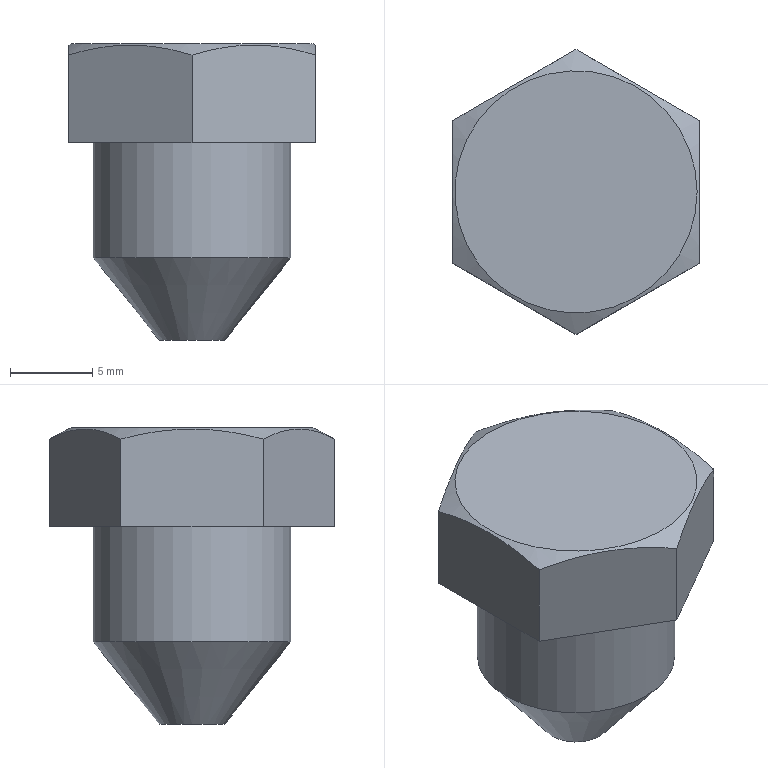Part | STEP file | 1-46.7 | 1 solid | 12 faces | box 15 x 17.321 x 18 mm | volume 2228 mm3 | plane 9 | cone 2 | cylinder 1 | commonest cylinder face diameters 12 x1
STEP:
#1=CARTESIAN_POINT('',(0.,0.,0.));
#2=DIRECTION('',(0.,0.,1.));
#3=DIRECTION('',(1.,0.,0.));
#4=AXIS2_PLACEMENT_3D('',#1,#2,#3);
#5=CARTESIAN_POINT('',(-7.5,-4.33,0.));
#6=VERTEX_POINT('',#5);
#7=CARTESIAN_POINT('',(-7.5,4.33,0.));
#8=VERTEX_POINT('',#7);
#9=CARTESIAN_POINT('',(-7.5,-4.33,0.));
#10=DIRECTION('',(0.,1.,0.));
#11=VECTOR('',#10,1.);
#12=LINE('',#9,#11);
#13=CARTESIAN_POINT('',(1.16,0.,0.));
#14=DIRECTION('',(0.,0.,-1.));
#15=DIRECTION('',(1.,0.,0.));
#16=AXIS2_PLACEMENT_3D('',#13,#14,#15);
#17=PLANE('',#16);
#18=CARTESIAN_POINT('',(-8.66,4.33));
#19=DIRECTION('',(0.,-1.));
#20=VECTOR('',#19,1.);
#21=LINE('',#18,#20);
#22=(GEOMETRIC_REPRESENTATION_CONTEXT(2)PARAMETRIC_REPRESENTATION_CONTEXT()REPRESENTATION_CONTEXT('',''));
#23=DEFINITIONAL_REPRESENTATION('',(#21),#22);
#24=PCURVE('',#17,#23);
#25=CARTESIAN_POINT('',(-7.5,0.,3.));
#26=DIRECTION('',(1.,0.,0.));
#27=DIRECTION('',(0.,1.,0.));
#28=AXIS2_PLACEMENT_3D('',#25,#26,#27);
#29=PLANE('',#28);
#30=CARTESIAN_POINT('',(-4.33,-3.));
#31=DIRECTION('',(1.,0.));
#32=VECTOR('',#31,1.);
#33=LINE('',#30,#32);
#34=(GEOMETRIC_REPRESENTATION_CONTEXT(2)PARAMETRIC_REPRESENTATION_CONTEXT()REPRESENTATION_CONTEXT('',''));
#35=DEFINITIONAL_REPRESENTATION('',(#33),#34);
#36=PCURVE('',#29,#35);
#37=SURFACE_CURVE('',#12,(#24,#36),.PCURVE_S1.);
#38=EDGE_CURVE('',#6,#8,#37,.T.);
#39=ORIENTED_EDGE('',*,*,#38,.T.);
#40=CARTESIAN_POINT('',(0.,8.66,0.));
#41=VERTEX_POINT('',#40);
#42=CARTESIAN_POINT('',(-7.5,4.33,0.));
#43=DIRECTION('',(0.866,0.5,0.));
#44=VECTOR('',#43,1.);
#45=LINE('',#42,#44);
#46=CARTESIAN_POINT('',(-8.66,-4.33));
#47=DIRECTION('',(0.866,-0.5));
#48=VECTOR('',#47,1.);
#49=LINE('',#46,#48);
#50=(GEOMETRIC_REPRESENTATION_CONTEXT(2)PARAMETRIC_REPRESENTATION_CONTEXT()REPRESENTATION_CONTEXT('',''));
#51=DEFINITIONAL_REPRESENTATION('',(#49),#50);
#52=PCURVE('',#17,#51);
#53=CARTESIAN_POINT('',(-3.75,6.495,3.));
#54=DIRECTION('',(0.5,-0.866,0.));
#55=DIRECTION('',(0.866,0.5,0.));
#56=AXIS2_PLACEMENT_3D('',#53,#54,#55);
#57=PLANE('',#56);
#58=CARTESIAN_POINT('',(-4.33,-3.));
#59=DIRECTION('',(1.,0.));
#60=VECTOR('',#59,1.);
#61=LINE('',#58,#60);
#62=(GEOMETRIC_REPRESENTATION_CONTEXT(2)PARAMETRIC_REPRESENTATION_CONTEXT()REPRESENTATION_CONTEXT('',''));
#63=DEFINITIONAL_REPRESENTATION('',(#61),#62);
#64=PCURVE('',#57,#63);
#65=SURFACE_CURVE('',#45,(#52,#64),.PCURVE_S1.);
#66=EDGE_CURVE('',#8,#41,#65,.T.);
#67=ORIENTED_EDGE('',*,*,#66,.T.);
#68=CARTESIAN_POINT('',(7.5,4.33,0.));
#69=VERTEX_POINT('',#68);
#70=CARTESIAN_POINT('',(0.,8.66,0.));
#71=DIRECTION('',(0.866,-0.5,0.));
#72=VECTOR('',#71,1.);
#73=LINE('',#70,#72);
#74=CARTESIAN_POINT('',(-1.16,-8.66));
#75=DIRECTION('',(0.866,0.5));
#76=VECTOR('',#75,1.);
#77=LINE('',#74,#76);
#78=(GEOMETRIC_REPRESENTATION_CONTEXT(2)PARAMETRIC_REPRESENTATION_CONTEXT()REPRESENTATION_CONTEXT('',''));
#79=DEFINITIONAL_REPRESENTATION('',(#77),#78);
#80=PCURVE('',#17,#79);
#81=CARTESIAN_POINT('',(3.75,6.495,3.));
#82=DIRECTION('',(-0.5,-0.866,0.));
#83=DIRECTION('',(0.866,-0.5,0.));
#84=AXIS2_PLACEMENT_3D('',#81,#82,#83);
#85=PLANE('',#84);
#86=CARTESIAN_POINT('',(-4.33,-3.));
#87=DIRECTION('',(1.,0.));
#88=VECTOR('',#87,1.);
#89=LINE('',#86,#88);
#90=(GEOMETRIC_REPRESENTATION_CONTEXT(2)PARAMETRIC_REPRESENTATION_CONTEXT()REPRESENTATION_CONTEXT('',''));
#91=DEFINITIONAL_REPRESENTATION('',(#89),#90);
#92=PCURVE('',#85,#91);
#93=SURFACE_CURVE('',#73,(#80,#92),.PCURVE_S1.);
#94=EDGE_CURVE('',#41,#69,#93,.T.);
#95=ORIENTED_EDGE('',*,*,#94,.T.);
#96=CARTESIAN_POINT('',(7.5,-4.33,0.));
#97=VERTEX_POINT('',#96);
#98=CARTESIAN_POINT('',(7.5,4.33,0.));
#99=DIRECTION('',(0.,-1.,0.));
#100=VECTOR('',#99,1.);
#101=LINE('',#98,#100);
#102=CARTESIAN_POINT('',(6.34,-4.33));
#103=DIRECTION('',(0.,1.));
#104=VECTOR('',#103,1.);
#105=LINE('',#102,#104);
#106=(GEOMETRIC_REPRESENTATION_CONTEXT(2)PARAMETRIC_REPRESENTATION_CONTEXT()REPRESENTATION_CONTEXT('',''));
#107=DEFINITIONAL_REPRESENTATION('',(#105),#106);
#108=PCURVE('',#17,#107);
#109=CARTESIAN_POINT('',(7.5,0.,3.));
#110=DIRECTION('',(-1.,0.,0.));
#111=DIRECTION('',(0.,-1.,0.));
#112=AXIS2_PLACEMENT_3D('',#109,#110,#111);
#113=PLANE('',#112);
#114=CARTESIAN_POINT('',(-4.33,-3.));
#115=DIRECTION('',(1.,0.));
#116=VECTOR('',#115,1.);
#117=LINE('',#114,#116);
#118=(GEOMETRIC_REPRESENTATION_CONTEXT(2)PARAMETRIC_REPRESENTATION_CONTEXT()REPRESENTATION_CONTEXT('',''));
#119=DEFINITIONAL_REPRESENTATION('',(#117),#118);
#120=PCURVE('',#113,#119);
#121=SURFACE_CURVE('',#101,(#108,#120),.PCURVE_S1.);
#122=EDGE_CURVE('',#69,#97,#121,.T.);
#123=ORIENTED_EDGE('',*,*,#122,.T.);
#124=CARTESIAN_POINT('',(0.,-8.66,0.));
#125=VERTEX_POINT('',#124);
#126=CARTESIAN_POINT('',(7.5,-4.33,0.));
#127=DIRECTION('',(-0.866,-0.5,0.));
#128=VECTOR('',#127,1.);
#129=LINE('',#126,#128);
#130=CARTESIAN_POINT('',(6.34,4.33));
#131=DIRECTION('',(-0.866,0.5));
#132=VECTOR('',#131,1.);
#133=LINE('',#130,#132);
#134=(GEOMETRIC_REPRESENTATION_CONTEXT(2)PARAMETRIC_REPRESENTATION_CONTEXT()REPRESENTATION_CONTEXT('',''));
#135=DEFINITIONAL_REPRESENTATION('',(#133),#134);
#136=PCURVE('',#17,#135);
#137=CARTESIAN_POINT('',(3.75,-6.495,3.));
#138=DIRECTION('',(-0.5,0.866,0.));
#139=DIRECTION('',(-0.866,-0.5,0.));
#140=AXIS2_PLACEMENT_3D('',#137,#138,#139);
#141=PLANE('',#140);
#142=CARTESIAN_POINT('',(-4.33,-3.));
#143=DIRECTION('',(1.,0.));
#144=VECTOR('',#143,1.);
#145=LINE('',#142,#144);
#146=(GEOMETRIC_REPRESENTATION_CONTEXT(2)PARAMETRIC_REPRESENTATION_CONTEXT()REPRESENTATION_CONTEXT('',''));
#147=DEFINITIONAL_REPRESENTATION('',(#145),#146);
#148=PCURVE('',#141,#147);
#149=SURFACE_CURVE('',#129,(#136,#148),.PCURVE_S1.);
#150=EDGE_CURVE('',#97,#125,#149,.T.);
#151=ORIENTED_EDGE('',*,*,#150,.T.);
#152=CARTESIAN_POINT('',(0.,-8.66,0.));
#153=DIRECTION('',(-0.866,0.5,0.));
#154=VECTOR('',#153,1.);
#155=LINE('',#152,#154);
#156=CARTESIAN_POINT('',(-1.16,8.66));
#157=DIRECTION('',(-0.866,-0.5));
#158=VECTOR('',#157,1.);
#159=LINE('',#156,#158);
#160=(GEOMETRIC_REPRESENTATION_CONTEXT(2)PARAMETRIC_REPRESENTATION_CONTEXT()REPRESENTATION_CONTEXT('',''));
#161=DEFINITIONAL_REPRESENTATION('',(#159),#160);
#162=PCURVE('',#17,#161);
#163=CARTESIAN_POINT('',(-3.75,-6.495,3.));
#164=DIRECTION('',(0.5,0.866,0.));
#165=DIRECTION('',(-0.866,0.5,0.));
#166=AXIS2_PLACEMENT_3D('',#163,#164,#165);
#167=PLANE('',#166);
#168=CARTESIAN_POINT('',(-4.33,-3.));
#169=DIRECTION('',(1.,0.));
#170=VECTOR('',#169,1.);
#171=LINE('',#168,#170);
#172=(GEOMETRIC_REPRESENTATION_CONTEXT(2)PARAMETRIC_REPRESENTATION_CONTEXT()REPRESENTATION_CONTEXT('',''));
#173=DEFINITIONAL_REPRESENTATION('',(#171),#172);
#174=PCURVE('',#167,#173);
#175=SURFACE_CURVE('',#155,(#162,#174),.PCURVE_S1.);
#176=EDGE_CURVE('',#125,#6,#175,.T.);
#177=ORIENTED_EDGE('',*,*,#176,.T.);
#178=EDGE_LOOP('',(#39,#67,#95,#123,#151,#177));
#179=FACE_BOUND('',#178,.T.);
#180=CARTESIAN_POINT('',(0.,6.,0.));
#181=VERTEX_POINT('',#180);
#182=CARTESIAN_POINT('',(0.,0.,0.));
#183=DIRECTION('',(0.,0.,1.));
#184=DIRECTION('',(0.,1.,0.));
#185=AXIS2_PLACEMENT_3D('',#182,#183,#184);
#186=CIRCLE('',#185,6.);
#187=CARTESIAN_POINT('',(-1.16,-6.));
#188=CARTESIAN_POINT('',(-11.553,-6.));
#189=CARTESIAN_POINT('',(-6.356,3.));
#190=CARTESIAN_POINT('',(-1.16,12.));
#191=CARTESIAN_POINT('',(4.036,3.));
#192=CARTESIAN_POINT('',(9.232,-6.));
#193=CARTESIAN_POINT('',(-1.16,-6.));
#194=(BOUNDED_CURVE()B_SPLINE_CURVE(2,(#187,#188,#189,#190,#191,#192,#193),.UNSPECIFIED.,.T.,.F.)B_SPLINE_CURVE_WITH_KNOTS((1,2,2,2,2,1),(-2.094,0.,2.094,4.189,6.283,8.378),.UNSPECIFIED.)CURVE()GEOMETRIC_REPRESENTATION_ITEM()RATIONAL_B_SPLINE_CURVE((1.,0.5,1.,0.5,1.,0.5,1.))REPRESENTATION_ITEM(''));
#195=(GEOMETRIC_REPRESENTATION_CONTEXT(2)PARAMETRIC_REPRESENTATION_CONTEXT()REPRESENTATION_CONTEXT('',''));
#196=DEFINITIONAL_REPRESENTATION('',(#194),#195);
#197=PCURVE('',#17,#196);
#198=CARTESIAN_POINT('',(0.,0.,0.));
#199=DIRECTION('',(0.,0.,-1.));
#200=DIRECTION('',(0.,1.,0.));
#201=AXIS2_PLACEMENT_3D('',#198,#199,#200);
#202=CYLINDRICAL_SURFACE('',#201,6.);
#203=CARTESIAN_POINT('',(6.283,0.));
#204=DIRECTION('',(-1.,0.));
#205=VECTOR('',#204,1.);
#206=LINE('',#203,#205);
#207=(GEOMETRIC_REPRESENTATION_CONTEXT(2)PARAMETRIC_REPRESENTATION_CONTEXT()REPRESENTATION_CONTEXT('',''));
#208=DEFINITIONAL_REPRESENTATION('',(#206),#207);
#209=PCURVE('',#202,#208);
#210=SURFACE_CURVE('',#186,(#197,#209),.PCURVE_S1.);
#211=EDGE_CURVE('',#181,#181,#210,.T.);
#212=ORIENTED_EDGE('',*,*,#211,.T.);
#213=EDGE_LOOP('',(#212));
#214=FACE_BOUND('',#213,.T.);
#215=ADVANCED_FACE('',(#179,#214),#17,.T.);
#216=CARTESIAN_POINT('',(0.,6.,-7.));
#217=VERTEX_POINT('',#216);
#218=CARTESIAN_POINT('',(0.,6.,0.));
#219=DIRECTION('',(0.,0.,-1.));
#220=VECTOR('',#219,1.);
#221=LINE('',#218,#220);
#222=CARTESIAN_POINT('',(6.283,0.));
#223=DIRECTION('',(0.,1.));
#224=VECTOR('',#223,1.);
#225=LINE('',#222,#224);
#226=(GEOMETRIC_REPRESENTATION_CONTEXT(2)PARAMETRIC_REPRESENTATION_CONTEXT()REPRESENTATION_CONTEXT('',''));
#227=DEFINITIONAL_REPRESENTATION('',(#225),#226);
#228=PCURVE('',#202,#227);
#229=CARTESIAN_POINT('',(0.,0.));
#230=DIRECTION('',(0.,1.));
#231=VECTOR('',#230,1.);
#232=LINE('',#229,#231);
#233=(GEOMETRIC_REPRESENTATION_CONTEXT(2)PARAMETRIC_REPRESENTATION_CONTEXT()REPRESENTATION_CONTEXT('',''));
#234=DEFINITIONAL_REPRESENTATION('',(#232),#233);
#235=PCURVE('',#202,#234);
#236=SEAM_CURVE('',#221,(#228,#235),.PCURVE_S1.);
#237=EDGE_CURVE('',#181,#217,#236,.T.);
#238=ORIENTED_EDGE('',*,*,#237,.T.);
#239=CARTESIAN_POINT('',(6.,0.,-7.));
#240=VERTEX_POINT('',#239);
#241=CARTESIAN_POINT('',(0.,0.,-7.));
#242=DIRECTION('',(0.,0.,1.));
#243=DIRECTION('',(0.,1.,0.));
#244=AXIS2_PLACEMENT_3D('',#241,#242,#243);
#245=CIRCLE('',#244,6.);
#246=CARTESIAN_POINT('',(6.283,7.));
#247=DIRECTION('',(-1.,0.));
#248=VECTOR('',#247,1.);
#249=LINE('',#246,#248);
#250=(GEOMETRIC_REPRESENTATION_CONTEXT(2)PARAMETRIC_REPRESENTATION_CONTEXT()REPRESENTATION_CONTEXT('',''));
#251=DEFINITIONAL_REPRESENTATION('',(#249),#250);
#252=PCURVE('',#202,#251);
#253=CARTESIAN_POINT('',(0.,0.,-12.));
#254=DIRECTION('',(0.,0.,1.));
#255=DIRECTION('',(1.,0.,0.));
#256=AXIS2_PLACEMENT_3D('',#253,#254,#255);
#257=CONICAL_SURFACE('',#256,2.,0.6747);
#258=CARTESIAN_POINT('',(1.571,5.));
#259=DIRECTION('',(1.,0.));
#260=VECTOR('',#259,1.);
#261=LINE('',#258,#260);
#262=(GEOMETRIC_REPRESENTATION_CONTEXT(2)PARAMETRIC_REPRESENTATION_CONTEXT()REPRESENTATION_CONTEXT('',''));
#263=DEFINITIONAL_REPRESENTATION('',(#261),#262);
#264=PCURVE('',#257,#263);
#265=SURFACE_CURVE('',#245,(#252,#264),.PCURVE_S1.);
#266=EDGE_CURVE('',#217,#240,#265,.T.);
#267=ORIENTED_EDGE('',*,*,#266,.T.);
#268=CARTESIAN_POINT('',(0.,0.,-7.));
#269=DIRECTION('',(0.,0.,1.));
#270=DIRECTION('',(1.,0.,0.));
#271=AXIS2_PLACEMENT_3D('',#268,#269,#270);
#272=CIRCLE('',#271,6.);
#273=CARTESIAN_POINT('',(1.571,7.));
#274=DIRECTION('',(-1.,0.));
#275=VECTOR('',#274,1.);
#276=LINE('',#273,#275);
#277=(GEOMETRIC_REPRESENTATION_CONTEXT(2)PARAMETRIC_REPRESENTATION_CONTEXT()REPRESENTATION_CONTEXT('',''));
#278=DEFINITIONAL_REPRESENTATION('',(#276),#277);
#279=PCURVE('',#202,#278);
#280=CARTESIAN_POINT('',(0.,5.));
#281=DIRECTION('',(1.,0.));
#282=VECTOR('',#281,1.);
#283=LINE('',#280,#282);
#284=(GEOMETRIC_REPRESENTATION_CONTEXT(2)PARAMETRIC_REPRESENTATION_CONTEXT()REPRESENTATION_CONTEXT('',''));
#285=DEFINITIONAL_REPRESENTATION('',(#283),#284);
#286=PCURVE('',#257,#285);
#287=SURFACE_CURVE('',#272,(#279,#286),.PCURVE_S1.);
#288=EDGE_CURVE('',#240,#217,#287,.T.);
#289=ORIENTED_EDGE('',*,*,#288,.T.);
#290=ORIENTED_EDGE('',*,*,#237,.F.);
#291=ORIENTED_EDGE('',*,*,#211,.F.);
#292=EDGE_LOOP('',(#238,#267,#289,#290,#291));
#293=FACE_BOUND('',#292,.T.);
#294=ADVANCED_FACE('',(#293),#202,.T.);
#295=CARTESIAN_POINT('',(2.,0.,-12.));
#296=VERTEX_POINT('',#295);
#297=CARTESIAN_POINT('',(0.,0.,-12.));
#298=DIRECTION('',(0.,0.,1.));
#299=DIRECTION('',(1.,0.,0.));
#300=AXIS2_PLACEMENT_3D('',#297,#298,#299);
#301=CIRCLE('',#300,2.);
#302=CARTESIAN_POINT('',(0.,0.));
#303=DIRECTION('',(1.,0.));
#304=VECTOR('',#303,1.);
#305=LINE('',#302,#304);
#306=(GEOMETRIC_REPRESENTATION_CONTEXT(2)PARAMETRIC_REPRESENTATION_CONTEXT()REPRESENTATION_CONTEXT('',''));
#307=DEFINITIONAL_REPRESENTATION('',(#305),#306);
#308=PCURVE('',#257,#307);
#309=CARTESIAN_POINT('',(0.,0.,-12.));
#310=DIRECTION('',(0.,0.,1.));
#311=DIRECTION('',(1.,0.,0.));
#312=AXIS2_PLACEMENT_3D('',#309,#310,#311);
#313=PLANE('',#312);
#314=CARTESIAN_POINT('',(0.,0.));
#315=DIRECTION('',(1.,0.));
#316=AXIS2_PLACEMENT_2D('',#314,#315);
#317=CIRCLE('',#316,2.);
#318=(GEOMETRIC_REPRESENTATION_CONTEXT(2)PARAMETRIC_REPRESENTATION_CONTEXT()REPRESENTATION_CONTEXT('',''));
#319=DEFINITIONAL_REPRESENTATION('',(#317),#318);
#320=PCURVE('',#313,#319);
#321=SURFACE_CURVE('',#301,(#308,#320),.PCURVE_S1.);
#322=EDGE_CURVE('',#296,#296,#321,.T.);
#323=ORIENTED_EDGE('',*,*,#322,.T.);
#324=CARTESIAN_POINT('',(2.,0.,-12.));
#325=DIRECTION('',(0.6247,0.,0.7809));
#326=VECTOR('',#325,1.);
#327=LINE('',#324,#326);
#328=CARTESIAN_POINT('',(6.283,0.));
#329=DIRECTION('',(0.,1.));
#330=VECTOR('',#329,1.);
#331=LINE('',#328,#330);
#332=(GEOMETRIC_REPRESENTATION_CONTEXT(2)PARAMETRIC_REPRESENTATION_CONTEXT()REPRESENTATION_CONTEXT('',''));
#333=DEFINITIONAL_REPRESENTATION('',(#331),#332);
#334=PCURVE('',#257,#333);
#335=CARTESIAN_POINT('',(0.,0.));
#336=DIRECTION('',(0.,1.));
#337=VECTOR('',#336,1.);
#338=LINE('',#335,#337);
#339=(GEOMETRIC_REPRESENTATION_CONTEXT(2)PARAMETRIC_REPRESENTATION_CONTEXT()REPRESENTATION_CONTEXT('',''));
#340=DEFINITIONAL_REPRESENTATION('',(#338),#339);
#341=PCURVE('',#257,#340);
#342=SEAM_CURVE('',#327,(#334,#341),.PCURVE_S1.);
#343=EDGE_CURVE('',#296,#240,#342,.T.);
#344=ORIENTED_EDGE('',*,*,#343,.T.);
#345=ORIENTED_EDGE('',*,*,#266,.F.);
#346=ORIENTED_EDGE('',*,*,#288,.F.);
#347=ORIENTED_EDGE('',*,*,#343,.F.);
#348=EDGE_LOOP('',(#323,#344,#345,#346,#347));
#349=FACE_BOUND('',#348,.T.);
#350=ADVANCED_FACE('',(#349),#257,.T.);
#351=ORIENTED_EDGE('',*,*,#322,.T.);
#352=EDGE_LOOP('',(#351));
#353=FACE_BOUND('',#352,.F.);
#354=ADVANCED_FACE('',(#353),#313,.F.);
#355=CARTESIAN_POINT('',(7.357,0.,6.));
#356=VERTEX_POINT('',#355);
#357=CARTESIAN_POINT('',(0.,0.,6.));
#358=DIRECTION('',(0.,0.,1.));
#359=DIRECTION('',(1.,0.,0.));
#360=AXIS2_PLACEMENT_3D('',#357,#358,#359);
#361=CIRCLE('',#360,7.357);
#362=CARTESIAN_POINT('',(1.16,0.,6.));
#363=DIRECTION('',(0.,0.,-1.));
#364=DIRECTION('',(1.,0.,0.));
#365=AXIS2_PLACEMENT_3D('',#362,#363,#364);
#366=PLANE('',#365);
#367=CARTESIAN_POINT('',(6.197,0.));
#368=CARTESIAN_POINT('',(6.197,-12.743));
#369=CARTESIAN_POINT('',(-4.839,-6.371));
#370=CARTESIAN_POINT('',(-15.874,0.));
#371=CARTESIAN_POINT('',(-4.839,6.371));
#372=CARTESIAN_POINT('',(6.197,12.743));
#373=CARTESIAN_POINT('',(6.197,0.));
#374=(BOUNDED_CURVE()B_SPLINE_CURVE(2,(#367,#368,#369,#370,#371,#372,#373),.UNSPECIFIED.,.T.,.F.)B_SPLINE_CURVE_WITH_KNOTS((1,2,2,2,2,1),(-2.094,0.,2.094,4.189,6.283,8.378),.UNSPECIFIED.)CURVE()GEOMETRIC_REPRESENTATION_ITEM()RATIONAL_B_SPLINE_CURVE((1.,0.5,1.,0.5,1.,0.5,1.))REPRESENTATION_ITEM(''));
#375=(GEOMETRIC_REPRESENTATION_CONTEXT(2)PARAMETRIC_REPRESENTATION_CONTEXT()REPRESENTATION_CONTEXT('',''));
#376=DEFINITIONAL_REPRESENTATION('',(#374),#375);
#377=PCURVE('',#366,#376);
#378=CARTESIAN_POINT('',(0.,0.,6.));
#379=DIRECTION('',(0.,0.,-1.));
#380=DIRECTION('',(1.,0.,0.));
#381=AXIS2_PLACEMENT_3D('',#378,#379,#380);
#382=CONICAL_SURFACE('',#381,7.357,1.09);
#383=CARTESIAN_POINT('',(6.283,0.));
#384=DIRECTION('',(-1.,0.));
#385=VECTOR('',#384,1.);
#386=LINE('',#383,#385);
#387=(GEOMETRIC_REPRESENTATION_CONTEXT(2)PARAMETRIC_REPRESENTATION_CONTEXT()REPRESENTATION_CONTEXT('',''));
#388=DEFINITIONAL_REPRESENTATION('',(#386),#387);
#389=PCURVE('',#382,#388);
#390=SURFACE_CURVE('',#361,(#377,#389),.PCURVE_S1.);
#391=EDGE_CURVE('',#356,#356,#390,.T.);
#392=ORIENTED_EDGE('',*,*,#391,.F.);
#393=EDGE_LOOP('',(#392));
#394=FACE_BOUND('',#393,.F.);
#395=ADVANCED_FACE('',(#394),#366,.F.);
#396=ORIENTED_EDGE('',*,*,#38,.T.);
#397=CARTESIAN_POINT('',(-7.5,4.33,5.32));
#398=VERTEX_POINT('',#397);
#399=CARTESIAN_POINT('',(-7.5,4.33,0.));
#400=DIRECTION('',(0.,0.,1.));
#401=VECTOR('',#400,1.);
#402=LINE('',#399,#401);
#403=CARTESIAN_POINT('',(4.33,-3.));
#404=DIRECTION('',(0.,1.));
#405=VECTOR('',#404,1.);
#406=LINE('',#403,#405);
#407=(GEOMETRIC_REPRESENTATION_CONTEXT(2)PARAMETRIC_REPRESENTATION_CONTEXT()REPRESENTATION_CONTEXT('',''));
#408=DEFINITIONAL_REPRESENTATION('',(#406),#407);
#409=PCURVE('',#29,#408);
#410=CARTESIAN_POINT('',(-4.33,-3.));
#411=DIRECTION('',(0.,1.));
#412=VECTOR('',#411,1.);
#413=LINE('',#410,#412);
#414=(GEOMETRIC_REPRESENTATION_CONTEXT(2)PARAMETRIC_REPRESENTATION_CONTEXT()REPRESENTATION_CONTEXT('',''));
#415=DEFINITIONAL_REPRESENTATION('',(#413),#414);
#416=PCURVE('',#57,#415);
#417=SURFACE_CURVE('',#402,(#409,#416),.PCURVE_S1.);
#418=EDGE_CURVE('',#8,#398,#417,.T.);
#419=ORIENTED_EDGE('',*,*,#418,.T.);
#420=CARTESIAN_POINT('',(-7.5,-4.33,5.32));
#421=VERTEX_POINT('',#420);
#422=CARTESIAN_POINT('',(-7.5,4.33,5.32));
#423=CARTESIAN_POINT('',(-7.5,0.,6.45));
#424=CARTESIAN_POINT('',(-7.5,-4.33,5.32));
#425=(BOUNDED_CURVE()B_SPLINE_CURVE(2,(#422,#423,#424),.UNSPECIFIED.,.F.,.F.)B_SPLINE_CURVE_WITH_KNOTS((3,3),(0.,1.),.PIECEWISE_BEZIER_KNOTS.)CURVE()GEOMETRIC_REPRESENTATION_ITEM()RATIONAL_B_SPLINE_CURVE((1.631,1.883,1.631))REPRESENTATION_ITEM(''));
#426=CARTESIAN_POINT('',(4.33,2.32));
#427=CARTESIAN_POINT('',(0.,3.45));
#428=CARTESIAN_POINT('',(-4.33,2.32));
#429=(BOUNDED_CURVE()B_SPLINE_CURVE(2,(#426,#427,#428),.UNSPECIFIED.,.F.,.F.)B_SPLINE_CURVE_WITH_KNOTS((3,3),(0.,1.),.PIECEWISE_BEZIER_KNOTS.)CURVE()GEOMETRIC_REPRESENTATION_ITEM()RATIONAL_B_SPLINE_CURVE((1.631,1.883,1.631))REPRESENTATION_ITEM(''));
#430=(GEOMETRIC_REPRESENTATION_CONTEXT(2)PARAMETRIC_REPRESENTATION_CONTEXT()REPRESENTATION_CONTEXT('',''));
#431=DEFINITIONAL_REPRESENTATION('',(#429),#430);
#432=PCURVE('',#29,#431);
#433=CARTESIAN_POINT('',(3.665,0.6804));
#434=CARTESIAN_POINT('',(3.65,0.6409));
#435=CARTESIAN_POINT('',(3.62,0.5665));
#436=CARTESIAN_POINT('',(3.573,0.468));
#437=CARTESIAN_POINT('',(3.527,0.3819));
#438=CARTESIAN_POINT('',(3.479,0.3074));
#439=CARTESIAN_POINT('',(3.432,0.2439));
#440=CARTESIAN_POINT('',(3.384,0.1909));
#441=CARTESIAN_POINT('',(3.336,0.1481));
#442=CARTESIAN_POINT('',(3.288,0.1151));
#443=CARTESIAN_POINT('',(3.239,0.09176));
#444=CARTESIAN_POINT('',(3.19,0.07779));
#445=CARTESIAN_POINT('',(3.142,0.07315));
#446=CARTESIAN_POINT('',(3.093,0.07779));
#447=CARTESIAN_POINT('',(3.044,0.09176));
#448=CARTESIAN_POINT('',(2.996,0.1151));
#449=CARTESIAN_POINT('',(2.947,0.1481));
#450=CARTESIAN_POINT('',(2.899,0.1909));
#451=CARTESIAN_POINT('',(2.851,0.2439));
#452=CARTESIAN_POINT('',(2.804,0.3074));
#453=CARTESIAN_POINT('',(2.757,0.3819));
#454=CARTESIAN_POINT('',(2.71,0.468));
#455=CARTESIAN_POINT('',(2.664,0.5665));
#456=CARTESIAN_POINT('',(2.633,0.6409));
#457=CARTESIAN_POINT('',(2.618,0.6804));
#458=B_SPLINE_CURVE_WITH_KNOTS('',3,(#433,#434,#435,#436,#437,#438,#439,#440,#441,#442,#443,#444,#445,#446,#447,#448,#449,#450,#451,#452,#453,#454,#455,#456,#457),.UNSPECIFIED.,.F.,.F.,(4,1,1,1,1,1,1,1,1,1,1,1,1,1,1,1,1,1,1,1,1,1,4),(0.,0.04545,0.09091,0.1364,0.1818,0.2273,0.2727,0.3182,0.3636,0.4091,0.4545,0.5,0.5455,0.5909,0.6364,0.6818,0.7273,0.7727,0.8182,0.8636,0.9091,0.9545,1.),.QUASI_UNIFORM_KNOTS.);
#459=(GEOMETRIC_REPRESENTATION_CONTEXT(2)PARAMETRIC_REPRESENTATION_CONTEXT()REPRESENTATION_CONTEXT('',''));
#460=DEFINITIONAL_REPRESENTATION('',(#458),#459);
#461=PCURVE('',#382,#460);
#462=SURFACE_CURVE('',#425,(#432,#461),.PCURVE_S1.);
#463=EDGE_CURVE('',#398,#421,#462,.T.);
#464=ORIENTED_EDGE('',*,*,#463,.T.);
#465=CARTESIAN_POINT('',(-7.5,-4.33,0.));
#466=DIRECTION('',(0.,0.,1.));
#467=VECTOR('',#466,1.);
#468=LINE('',#465,#467);
#469=CARTESIAN_POINT('',(-4.33,-3.));
#470=DIRECTION('',(0.,1.));
#471=VECTOR('',#470,1.);
#472=LINE('',#469,#471);
#473=(GEOMETRIC_REPRESENTATION_CONTEXT(2)PARAMETRIC_REPRESENTATION_CONTEXT()REPRESENTATION_CONTEXT('',''));
#474=DEFINITIONAL_REPRESENTATION('',(#472),#473);
#475=PCURVE('',#29,#474);
#476=CARTESIAN_POINT('',(4.33,-3.));
#477=DIRECTION('',(0.,1.));
#478=VECTOR('',#477,1.);
#479=LINE('',#476,#478);
#480=(GEOMETRIC_REPRESENTATION_CONTEXT(2)PARAMETRIC_REPRESENTATION_CONTEXT()REPRESENTATION_CONTEXT('',''));
#481=DEFINITIONAL_REPRESENTATION('',(#479),#480);
#482=PCURVE('',#167,#481);
#483=SURFACE_CURVE('',#468,(#475,#482),.PCURVE_S1.);
#484=EDGE_CURVE('',#6,#421,#483,.T.);
#485=ORIENTED_EDGE('',*,*,#484,.F.);
#486=EDGE_LOOP('',(#396,#419,#464,#485));
#487=FACE_BOUND('',#486,.F.);
#488=ADVANCED_FACE('',(#487),#29,.F.);
#489=ORIENTED_EDGE('',*,*,#66,.T.);
#490=CARTESIAN_POINT('',(0.,8.66,5.32));
#491=VERTEX_POINT('',#490);
#492=CARTESIAN_POINT('',(0.,8.66,0.));
#493=DIRECTION('',(0.,0.,1.));
#494=VECTOR('',#493,1.);
#495=LINE('',#492,#494);
#496=CARTESIAN_POINT('',(4.33,-3.));
#497=DIRECTION('',(0.,1.));
#498=VECTOR('',#497,1.);
#499=LINE('',#496,#498);
#500=(GEOMETRIC_REPRESENTATION_CONTEXT(2)PARAMETRIC_REPRESENTATION_CONTEXT()REPRESENTATION_CONTEXT('',''));
#501=DEFINITIONAL_REPRESENTATION('',(#499),#500);
#502=PCURVE('',#57,#501);
#503=CARTESIAN_POINT('',(-4.33,-3.));
#504=DIRECTION('',(0.,1.));
#505=VECTOR('',#504,1.);
#506=LINE('',#503,#505);
#507=(GEOMETRIC_REPRESENTATION_CONTEXT(2)PARAMETRIC_REPRESENTATION_CONTEXT()REPRESENTATION_CONTEXT('',''));
#508=DEFINITIONAL_REPRESENTATION('',(#506),#507);
#509=PCURVE('',#85,#508);
#510=SURFACE_CURVE('',#495,(#502,#509),.PCURVE_S1.);
#511=EDGE_CURVE('',#41,#491,#510,.T.);
#512=ORIENTED_EDGE('',*,*,#511,.T.);
#513=CARTESIAN_POINT('',(0.,8.66,5.32));
#514=CARTESIAN_POINT('',(-3.75,6.495,6.45));
#515=CARTESIAN_POINT('',(-7.5,4.33,5.32));
#516=(BOUNDED_CURVE()B_SPLINE_CURVE(2,(#513,#514,#515),.UNSPECIFIED.,.F.,.F.)B_SPLINE_CURVE_WITH_KNOTS((3,3),(0.,1.),.PIECEWISE_BEZIER_KNOTS.)CURVE()GEOMETRIC_REPRESENTATION_ITEM()RATIONAL_B_SPLINE_CURVE((1.631,1.883,1.631))REPRESENTATION_ITEM(''));
#517=CARTESIAN_POINT('',(4.33,2.32));
#518=CARTESIAN_POINT('',(0.,3.45));
#519=CARTESIAN_POINT('',(-4.33,2.32));
#520=(BOUNDED_CURVE()B_SPLINE_CURVE(2,(#517,#518,#519),.UNSPECIFIED.,.F.,.F.)B_SPLINE_CURVE_WITH_KNOTS((3,3),(0.,1.),.PIECEWISE_BEZIER_KNOTS.)CURVE()GEOMETRIC_REPRESENTATION_ITEM()RATIONAL_B_SPLINE_CURVE((1.631,1.883,1.631))REPRESENTATION_ITEM(''));
#521=(GEOMETRIC_REPRESENTATION_CONTEXT(2)PARAMETRIC_REPRESENTATION_CONTEXT()REPRESENTATION_CONTEXT('',''));
#522=DEFINITIONAL_REPRESENTATION('',(#520),#521);
#523=PCURVE('',#57,#522);
#524=CARTESIAN_POINT('',(4.712,0.6804));
#525=CARTESIAN_POINT('',(4.697,0.6409));
#526=CARTESIAN_POINT('',(4.667,0.5665));
#527=CARTESIAN_POINT('',(4.621,0.468));
#528=CARTESIAN_POINT('',(4.574,0.3819));
#529=CARTESIAN_POINT('',(4.527,0.3074));
#530=CARTESIAN_POINT('',(4.479,0.2439));
#531=CARTESIAN_POINT('',(4.431,0.1909));
#532=CARTESIAN_POINT('',(4.383,0.1481));
#533=CARTESIAN_POINT('',(4.335,0.1151));
#534=CARTESIAN_POINT('',(4.286,0.09176));
#535=CARTESIAN_POINT('',(4.238,0.07779));
#536=CARTESIAN_POINT('',(4.189,0.07315));
#537=CARTESIAN_POINT('',(4.14,0.07779));
#538=CARTESIAN_POINT('',(4.091,0.09176));
#539=CARTESIAN_POINT('',(4.043,0.1151));
#540=CARTESIAN_POINT('',(3.994,0.1481));
#541=CARTESIAN_POINT('',(3.946,0.1909));
#542=CARTESIAN_POINT('',(3.898,0.2439));
#543=CARTESIAN_POINT('',(3.851,0.3074));
#544=CARTESIAN_POINT('',(3.804,0.3819));
#545=CARTESIAN_POINT('',(3.757,0.468));
#546=CARTESIAN_POINT('',(3.711,0.5665));
#547=CARTESIAN_POINT('',(3.68,0.6409));
#548=CARTESIAN_POINT('',(3.665,0.6804));
#549=B_SPLINE_CURVE_WITH_KNOTS('',3,(#524,#525,#526,#527,#528,#529,#530,#531,#532,#533,#534,#535,#536,#537,#538,#539,#540,#541,#542,#543,#544,#545,#546,#547,#548),.UNSPECIFIED.,.F.,.F.,(4,1,1,1,1,1,1,1,1,1,1,1,1,1,1,1,1,1,1,1,1,1,4),(0.,0.04545,0.09091,0.1364,0.1818,0.2273,0.2727,0.3182,0.3636,0.4091,0.4545,0.5,0.5455,0.5909,0.6364,0.6818,0.7273,0.7727,0.8182,0.8636,0.9091,0.9545,1.),.QUASI_UNIFORM_KNOTS.);
#550=(GEOMETRIC_REPRESENTATION_CONTEXT(2)PARAMETRIC_REPRESENTATION_CONTEXT()REPRESENTATION_CONTEXT('',''));
#551=DEFINITIONAL_REPRESENTATION('',(#549),#550);
#552=PCURVE('',#382,#551);
#553=SURFACE_CURVE('',#516,(#523,#552),.PCURVE_S1.);
#554=EDGE_CURVE('',#491,#398,#553,.T.);
#555=ORIENTED_EDGE('',*,*,#554,.T.);
#556=ORIENTED_EDGE('',*,*,#418,.F.);
#557=EDGE_LOOP('',(#489,#512,#555,#556));
#558=FACE_BOUND('',#557,.F.);
#559=ADVANCED_FACE('',(#558),#57,.F.);
#560=ORIENTED_EDGE('',*,*,#94,.T.);
#561=CARTESIAN_POINT('',(7.5,4.33,5.32));
#562=VERTEX_POINT('',#561);
#563=CARTESIAN_POINT('',(7.5,4.33,0.));
#564=DIRECTION('',(0.,0.,1.));
#565=VECTOR('',#564,1.);
#566=LINE('',#563,#565);
#567=CARTESIAN_POINT('',(4.33,-3.));
#568=DIRECTION('',(0.,1.));
#569=VECTOR('',#568,1.);
#570=LINE('',#567,#569);
#571=(GEOMETRIC_REPRESENTATION_CONTEXT(2)PARAMETRIC_REPRESENTATION_CONTEXT()REPRESENTATION_CONTEXT('',''));
#572=DEFINITIONAL_REPRESENTATION('',(#570),#571);
#573=PCURVE('',#85,#572);
#574=CARTESIAN_POINT('',(-4.33,-3.));
#575=DIRECTION('',(0.,1.));
#576=VECTOR('',#575,1.);
#577=LINE('',#574,#576);
#578=(GEOMETRIC_REPRESENTATION_CONTEXT(2)PARAMETRIC_REPRESENTATION_CONTEXT()REPRESENTATION_CONTEXT('',''));
#579=DEFINITIONAL_REPRESENTATION('',(#577),#578);
#580=PCURVE('',#113,#579);
#581=SURFACE_CURVE('',#566,(#573,#580),.PCURVE_S1.);
#582=EDGE_CURVE('',#69,#562,#581,.T.);
#583=ORIENTED_EDGE('',*,*,#582,.T.);
#584=CARTESIAN_POINT('',(7.5,4.33,5.32));
#585=CARTESIAN_POINT('',(3.75,6.495,6.45));
#586=CARTESIAN_POINT('',(0.,8.66,5.32));
#587=(BOUNDED_CURVE()B_SPLINE_CURVE(2,(#584,#585,#586),.UNSPECIFIED.,.F.,.F.)B_SPLINE_CURVE_WITH_KNOTS((3,3),(0.,1.),.PIECEWISE_BEZIER_KNOTS.)CURVE()GEOMETRIC_REPRESENTATION_ITEM()RATIONAL_B_SPLINE_CURVE((1.631,1.883,1.631))REPRESENTATION_ITEM(''));
#588=CARTESIAN_POINT('',(4.33,2.32));
#589=CARTESIAN_POINT('',(0.,3.45));
#590=CARTESIAN_POINT('',(-4.33,2.32));
#591=(BOUNDED_CURVE()B_SPLINE_CURVE(2,(#588,#589,#590),.UNSPECIFIED.,.F.,.F.)B_SPLINE_CURVE_WITH_KNOTS((3,3),(0.,1.),.PIECEWISE_BEZIER_KNOTS.)CURVE()GEOMETRIC_REPRESENTATION_ITEM()RATIONAL_B_SPLINE_CURVE((1.631,1.883,1.631))REPRESENTATION_ITEM(''));
#592=(GEOMETRIC_REPRESENTATION_CONTEXT(2)PARAMETRIC_REPRESENTATION_CONTEXT()REPRESENTATION_CONTEXT('',''));
#593=DEFINITIONAL_REPRESENTATION('',(#591),#592);
#594=PCURVE('',#85,#593);
#595=CARTESIAN_POINT('',(5.76,0.6804));
#596=CARTESIAN_POINT('',(5.744,0.6409));
#597=CARTESIAN_POINT('',(5.714,0.5665));
#598=CARTESIAN_POINT('',(5.668,0.468));
#599=CARTESIAN_POINT('',(5.621,0.3819));
#600=CARTESIAN_POINT('',(5.574,0.3074));
#601=CARTESIAN_POINT('',(5.526,0.2439));
#602=CARTESIAN_POINT('',(5.478,0.1909));
#603=CARTESIAN_POINT('',(5.43,0.1481));
#604=CARTESIAN_POINT('',(5.382,0.1151));
#605=CARTESIAN_POINT('',(5.333,0.09176));
#606=CARTESIAN_POINT('',(5.285,0.07779));
#607=CARTESIAN_POINT('',(5.236,0.07315));
#608=CARTESIAN_POINT('',(5.187,0.07779));
#609=CARTESIAN_POINT('',(5.139,0.09176));
#610=CARTESIAN_POINT('',(5.09,0.1151));
#611=CARTESIAN_POINT('',(5.042,0.1481));
#612=CARTESIAN_POINT('',(4.994,0.1909));
#613=CARTESIAN_POINT('',(4.946,0.2439));
#614=CARTESIAN_POINT('',(4.898,0.3074));
#615=CARTESIAN_POINT('',(4.851,0.3819));
#616=CARTESIAN_POINT('',(4.804,0.468));
#617=CARTESIAN_POINT('',(4.758,0.5665));
#618=CARTESIAN_POINT('',(4.728,0.6409));
#619=CARTESIAN_POINT('',(4.712,0.6804));
#620=B_SPLINE_CURVE_WITH_KNOTS('',3,(#595,#596,#597,#598,#599,#600,#601,#602,#603,#604,#605,#606,#607,#608,#609,#610,#611,#612,#613,#614,#615,#616,#617,#618,#619),.UNSPECIFIED.,.F.,.F.,(4,1,1,1,1,1,1,1,1,1,1,1,1,1,1,1,1,1,1,1,1,1,4),(0.,0.04545,0.09091,0.1364,0.1818,0.2273,0.2727,0.3182,0.3636,0.4091,0.4545,0.5,0.5455,0.5909,0.6364,0.6818,0.7273,0.7727,0.8182,0.8636,0.9091,0.9545,1.),.QUASI_UNIFORM_KNOTS.);
#621=(GEOMETRIC_REPRESENTATION_CONTEXT(2)PARAMETRIC_REPRESENTATION_CONTEXT()REPRESENTATION_CONTEXT('',''));
#622=DEFINITIONAL_REPRESENTATION('',(#620),#621);
#623=PCURVE('',#382,#622);
#624=SURFACE_CURVE('',#587,(#594,#623),.PCURVE_S1.);
#625=EDGE_CURVE('',#562,#491,#624,.T.);
#626=ORIENTED_EDGE('',*,*,#625,.T.);
#627=ORIENTED_EDGE('',*,*,#511,.F.);
#628=EDGE_LOOP('',(#560,#583,#626,#627));
#629=FACE_BOUND('',#628,.F.);
#630=ADVANCED_FACE('',(#629),#85,.F.);
#631=ORIENTED_EDGE('',*,*,#122,.T.);
#632=CARTESIAN_POINT('',(7.5,-4.33,5.32));
#633=VERTEX_POINT('',#632);
#634=CARTESIAN_POINT('',(7.5,-4.33,0.));
#635=DIRECTION('',(0.,0.,1.));
#636=VECTOR('',#635,1.);
#637=LINE('',#634,#636);
#638=CARTESIAN_POINT('',(4.33,-3.));
#639=DIRECTION('',(0.,1.));
#640=VECTOR('',#639,1.);
#641=LINE('',#638,#640);
#642=(GEOMETRIC_REPRESENTATION_CONTEXT(2)PARAMETRIC_REPRESENTATION_CONTEXT()REPRESENTATION_CONTEXT('',''));
#643=DEFINITIONAL_REPRESENTATION('',(#641),#642);
#644=PCURVE('',#113,#643);
#645=CARTESIAN_POINT('',(-4.33,-3.));
#646=DIRECTION('',(0.,1.));
#647=VECTOR('',#646,1.);
#648=LINE('',#645,#647);
#649=(GEOMETRIC_REPRESENTATION_CONTEXT(2)PARAMETRIC_REPRESENTATION_CONTEXT()REPRESENTATION_CONTEXT('',''));
#650=DEFINITIONAL_REPRESENTATION('',(#648),#649);
#651=PCURVE('',#141,#650);
#652=SURFACE_CURVE('',#637,(#644,#651),.PCURVE_S1.);
#653=EDGE_CURVE('',#97,#633,#652,.T.);
#654=ORIENTED_EDGE('',*,*,#653,.T.);
#655=CARTESIAN_POINT('',(7.5,0.,5.925));
#656=VERTEX_POINT('',#655);
#657=CARTESIAN_POINT('',(7.5,-4.33,5.32));
#658=CARTESIAN_POINT('',(7.5,-2.01,5.925));
#659=CARTESIAN_POINT('',(7.5,0.,5.925));
#660=(BOUNDED_CURVE()B_SPLINE_CURVE(2,(#657,#658,#659),.UNSPECIFIED.,.F.,.F.)B_SPLINE_CURVE_WITH_KNOTS((3,3),(0.,1.),.PIECEWISE_BEZIER_KNOTS.)CURVE()GEOMETRIC_REPRESENTATION_ITEM()RATIONAL_B_SPLINE_CURVE((1.631,1.757,1.757))REPRESENTATION_ITEM(''));
#661=CARTESIAN_POINT('',(4.33,2.32));
#662=CARTESIAN_POINT('',(2.01,2.925));
#663=CARTESIAN_POINT('',(0.,2.925));
#664=(BOUNDED_CURVE()B_SPLINE_CURVE(2,(#661,#662,#663),.UNSPECIFIED.,.F.,.F.)B_SPLINE_CURVE_WITH_KNOTS((3,3),(0.,1.),.PIECEWISE_BEZIER_KNOTS.)CURVE()GEOMETRIC_REPRESENTATION_ITEM()RATIONAL_B_SPLINE_CURVE((1.631,1.757,1.757))REPRESENTATION_ITEM(''));
#665=(GEOMETRIC_REPRESENTATION_CONTEXT(2)PARAMETRIC_REPRESENTATION_CONTEXT()REPRESENTATION_CONTEXT('',''));
#666=DEFINITIONAL_REPRESENTATION('',(#664),#665);
#667=PCURVE('',#113,#666);
#668=CARTESIAN_POINT('',(0.5236,0.6804));
#669=CARTESIAN_POINT('',(0.516,0.6606));
#670=CARTESIAN_POINT('',(0.5008,0.6223));
#671=CARTESIAN_POINT('',(0.4779,0.5681));
#672=CARTESIAN_POINT('',(0.4548,0.5172));
#673=CARTESIAN_POINT('',(0.4317,0.4695));
#674=CARTESIAN_POINT('',(0.4084,0.4249));
#675=CARTESIAN_POINT('',(0.3849,0.3833));
#676=CARTESIAN_POINT('',(0.3614,0.3446));
#677=CARTESIAN_POINT('',(0.3378,0.3087));
#678=CARTESIAN_POINT('',(0.3141,0.2756));
#679=CARTESIAN_POINT('',(0.2903,0.2452));
#680=CARTESIAN_POINT('',(0.2664,0.2174));
#681=CARTESIAN_POINT('',(0.2424,0.1922));
#682=CARTESIAN_POINT('',(0.2184,0.1695));
#683=CARTESIAN_POINT('',(0.1943,0.1493));
#684=CARTESIAN_POINT('',(0.1701,0.1316));
#685=CARTESIAN_POINT('',(0.1459,0.1163));
#686=CARTESIAN_POINT('',(0.1217,0.1035));
#687=CARTESIAN_POINT('',(0.09736,0.09293));
#688=CARTESIAN_POINT('',(0.07305,0.08478));
#689=CARTESIAN_POINT('',(0.04871,0.07896));
#690=CARTESIAN_POINT('',(0.02436,0.07547));
#691=CARTESIAN_POINT('',(0.00812,0.0747));
#692=CARTESIAN_POINT('',(0.,0.0747));
#693=B_SPLINE_CURVE_WITH_KNOTS('',3,(#668,#669,#670,#671,#672,#673,#674,#675,#676,#677,#678,#679,#680,#681,#682,#683,#684,#685,#686,#687,#688,#689,#690,#691,#692),.UNSPECIFIED.,.F.,.F.,(4,1,1,1,1,1,1,1,1,1,1,1,1,1,1,1,1,1,1,1,1,1,4),(0.,0.04545,0.09091,0.1364,0.1818,0.2273,0.2727,0.3182,0.3636,0.4091,0.4545,0.5,0.5455,0.5909,0.6364,0.6818,0.7273,0.7727,0.8182,0.8636,0.9091,0.9545,1.),.QUASI_UNIFORM_KNOTS.);
#694=(GEOMETRIC_REPRESENTATION_CONTEXT(2)PARAMETRIC_REPRESENTATION_CONTEXT()REPRESENTATION_CONTEXT('',''));
#695=DEFINITIONAL_REPRESENTATION('',(#693),#694);
#696=PCURVE('',#382,#695);
#697=SURFACE_CURVE('',#660,(#667,#696),.PCURVE_S1.);
#698=EDGE_CURVE('',#633,#656,#697,.T.);
#699=ORIENTED_EDGE('',*,*,#698,.T.);
#700=CARTESIAN_POINT('',(7.5,0.,5.925));
#701=CARTESIAN_POINT('',(7.5,2.01,5.925));
#702=CARTESIAN_POINT('',(7.5,4.33,5.32));
#703=(BOUNDED_CURVE()B_SPLINE_CURVE(2,(#700,#701,#702),.UNSPECIFIED.,.F.,.F.)B_SPLINE_CURVE_WITH_KNOTS((3,3),(0.,1.),.PIECEWISE_BEZIER_KNOTS.)CURVE()GEOMETRIC_REPRESENTATION_ITEM()RATIONAL_B_SPLINE_CURVE((1.757,1.757,1.631))REPRESENTATION_ITEM(''));
#704=CARTESIAN_POINT('',(0.,2.925));
#705=CARTESIAN_POINT('',(-2.01,2.925));
#706=CARTESIAN_POINT('',(-4.33,2.32));
#707=(BOUNDED_CURVE()B_SPLINE_CURVE(2,(#704,#705,#706),.UNSPECIFIED.,.F.,.F.)B_SPLINE_CURVE_WITH_KNOTS((3,3),(0.,1.),.PIECEWISE_BEZIER_KNOTS.)CURVE()GEOMETRIC_REPRESENTATION_ITEM()RATIONAL_B_SPLINE_CURVE((1.757,1.757,1.631))REPRESENTATION_ITEM(''));
#708=(GEOMETRIC_REPRESENTATION_CONTEXT(2)PARAMETRIC_REPRESENTATION_CONTEXT()REPRESENTATION_CONTEXT('',''));
#709=DEFINITIONAL_REPRESENTATION('',(#707),#708);
#710=PCURVE('',#113,#709);
#711=CARTESIAN_POINT('',(6.283,0.0747));
#712=CARTESIAN_POINT('',(6.275,0.0747));
#713=CARTESIAN_POINT('',(6.259,0.07547));
#714=CARTESIAN_POINT('',(6.234,0.07896));
#715=CARTESIAN_POINT('',(6.21,0.08478));
#716=CARTESIAN_POINT('',(6.186,0.09293));
#717=CARTESIAN_POINT('',(6.162,0.1035));
#718=CARTESIAN_POINT('',(6.137,0.1163));
#719=CARTESIAN_POINT('',(6.113,0.1316));
#720=CARTESIAN_POINT('',(6.089,0.1493));
#721=CARTESIAN_POINT('',(6.065,0.1695));
#722=CARTESIAN_POINT('',(6.041,0.1922));
#723=CARTESIAN_POINT('',(6.017,0.2174));
#724=CARTESIAN_POINT('',(5.993,0.2452));
#725=CARTESIAN_POINT('',(5.969,0.2756));
#726=CARTESIAN_POINT('',(5.945,0.3087));
#727=CARTESIAN_POINT('',(5.922,0.3446));
#728=CARTESIAN_POINT('',(5.898,0.3833));
#729=CARTESIAN_POINT('',(5.875,0.4249));
#730=CARTESIAN_POINT('',(5.852,0.4695));
#731=CARTESIAN_POINT('',(5.828,0.5172));
#732=CARTESIAN_POINT('',(5.805,0.5681));
#733=CARTESIAN_POINT('',(5.782,0.6223));
#734=CARTESIAN_POINT('',(5.767,0.6606));
#735=CARTESIAN_POINT('',(5.76,0.6804));
#736=B_SPLINE_CURVE_WITH_KNOTS('',3,(#711,#712,#713,#714,#715,#716,#717,#718,#719,#720,#721,#722,#723,#724,#725,#726,#727,#728,#729,#730,#731,#732,#733,#734,#735),.UNSPECIFIED.,.F.,.F.,(4,1,1,1,1,1,1,1,1,1,1,1,1,1,1,1,1,1,1,1,1,1,4),(0.,0.04545,0.09091,0.1364,0.1818,0.2273,0.2727,0.3182,0.3636,0.4091,0.4545,0.5,0.5455,0.5909,0.6364,0.6818,0.7273,0.7727,0.8182,0.8636,0.9091,0.9545,1.),.QUASI_UNIFORM_KNOTS.);
#737=(GEOMETRIC_REPRESENTATION_CONTEXT(2)PARAMETRIC_REPRESENTATION_CONTEXT()REPRESENTATION_CONTEXT('',''));
#738=DEFINITIONAL_REPRESENTATION('',(#736),#737);
#739=PCURVE('',#382,#738);
#740=SURFACE_CURVE('',#703,(#710,#739),.PCURVE_S1.);
#741=EDGE_CURVE('',#656,#562,#740,.T.);
#742=ORIENTED_EDGE('',*,*,#741,.T.);
#743=ORIENTED_EDGE('',*,*,#582,.F.);
#744=EDGE_LOOP('',(#631,#654,#699,#742,#743));
#745=FACE_BOUND('',#744,.F.);
#746=ADVANCED_FACE('',(#745),#113,.F.);
#747=ORIENTED_EDGE('',*,*,#150,.T.);
#748=CARTESIAN_POINT('',(0.,-8.66,5.32));
#749=VERTEX_POINT('',#748);
#750=CARTESIAN_POINT('',(0.,-8.66,0.));
#751=DIRECTION('',(0.,0.,1.));
#752=VECTOR('',#751,1.);
#753=LINE('',#750,#752);
#754=CARTESIAN_POINT('',(4.33,-3.));
#755=DIRECTION('',(0.,1.));
#756=VECTOR('',#755,1.);
#757=LINE('',#754,#756);
#758=(GEOMETRIC_REPRESENTATION_CONTEXT(2)PARAMETRIC_REPRESENTATION_CONTEXT()REPRESENTATION_CONTEXT('',''));
#759=DEFINITIONAL_REPRESENTATION('',(#757),#758);
#760=PCURVE('',#141,#759);
#761=CARTESIAN_POINT('',(-4.33,-3.));
#762=DIRECTION('',(0.,1.));
#763=VECTOR('',#762,1.);
#764=LINE('',#761,#763);
#765=(GEOMETRIC_REPRESENTATION_CONTEXT(2)PARAMETRIC_REPRESENTATION_CONTEXT()REPRESENTATION_CONTEXT('',''));
#766=DEFINITIONAL_REPRESENTATION('',(#764),#765);
#767=PCURVE('',#167,#766);
#768=SURFACE_CURVE('',#753,(#760,#767),.PCURVE_S1.);
#769=EDGE_CURVE('',#125,#749,#768,.T.);
#770=ORIENTED_EDGE('',*,*,#769,.T.);
#771=CARTESIAN_POINT('',(0.,-8.66,5.32));
#772=CARTESIAN_POINT('',(3.75,-6.495,6.45));
#773=CARTESIAN_POINT('',(7.5,-4.33,5.32));
#774=(BOUNDED_CURVE()B_SPLINE_CURVE(2,(#771,#772,#773),.UNSPECIFIED.,.F.,.F.)B_SPLINE_CURVE_WITH_KNOTS((3,3),(0.,1.),.PIECEWISE_BEZIER_KNOTS.)CURVE()GEOMETRIC_REPRESENTATION_ITEM()RATIONAL_B_SPLINE_CURVE((1.631,1.883,1.631))REPRESENTATION_ITEM(''));
#775=CARTESIAN_POINT('',(4.33,2.32));
#776=CARTESIAN_POINT('',(0.,3.45));
#777=CARTESIAN_POINT('',(-4.33,2.32));
#778=(BOUNDED_CURVE()B_SPLINE_CURVE(2,(#775,#776,#777),.UNSPECIFIED.,.F.,.F.)B_SPLINE_CURVE_WITH_KNOTS((3,3),(0.,1.),.PIECEWISE_BEZIER_KNOTS.)CURVE()GEOMETRIC_REPRESENTATION_ITEM()RATIONAL_B_SPLINE_CURVE((1.631,1.883,1.631))REPRESENTATION_ITEM(''));
#779=(GEOMETRIC_REPRESENTATION_CONTEXT(2)PARAMETRIC_REPRESENTATION_CONTEXT()REPRESENTATION_CONTEXT('',''));
#780=DEFINITIONAL_REPRESENTATION('',(#778),#779);
#781=PCURVE('',#141,#780);
#782=CARTESIAN_POINT('',(1.571,0.6804));
#783=CARTESIAN_POINT('',(1.556,0.6409));
#784=CARTESIAN_POINT('',(1.525,0.5665));
#785=CARTESIAN_POINT('',(1.479,0.468));
#786=CARTESIAN_POINT('',(1.432,0.3819));
#787=CARTESIAN_POINT('',(1.385,0.3074));
#788=CARTESIAN_POINT('',(1.338,0.2439));
#789=CARTESIAN_POINT('',(1.29,0.1909));
#790=CARTESIAN_POINT('',(1.241,0.1481));
#791=CARTESIAN_POINT('',(1.193,0.1151));
#792=CARTESIAN_POINT('',(1.145,0.09176));
#793=CARTESIAN_POINT('',(1.096,0.07779));
#794=CARTESIAN_POINT('',(1.047,0.07315));
#795=CARTESIAN_POINT('',(0.9985,0.07779));
#796=CARTESIAN_POINT('',(0.9498,0.09176));
#797=CARTESIAN_POINT('',(0.9013,0.1151));
#798=CARTESIAN_POINT('',(0.8529,0.1481));
#799=CARTESIAN_POINT('',(0.8048,0.1909));
#800=CARTESIAN_POINT('',(0.7569,0.2439));
#801=CARTESIAN_POINT('',(0.7094,0.3074));
#802=CARTESIAN_POINT('',(0.6622,0.3819));
#803=CARTESIAN_POINT('',(0.6155,0.468));
#804=CARTESIAN_POINT('',(0.5692,0.5665));
#805=CARTESIAN_POINT('',(0.5388,0.6409));
#806=CARTESIAN_POINT('',(0.5236,0.6804));
#807=B_SPLINE_CURVE_WITH_KNOTS('',3,(#782,#783,#784,#785,#786,#787,#788,#789,#790,#791,#792,#793,#794,#795,#796,#797,#798,#799,#800,#801,#802,#803,#804,#805,#806),.UNSPECIFIED.,.F.,.F.,(4,1,1,1,1,1,1,1,1,1,1,1,1,1,1,1,1,1,1,1,1,1,4),(0.,0.04545,0.09091,0.1364,0.1818,0.2273,0.2727,0.3182,0.3636,0.4091,0.4545,0.5,0.5455,0.5909,0.6364,0.6818,0.7273,0.7727,0.8182,0.8636,0.9091,0.9545,1.),.QUASI_UNIFORM_KNOTS.);
#808=(GEOMETRIC_REPRESENTATION_CONTEXT(2)PARAMETRIC_REPRESENTATION_CONTEXT()REPRESENTATION_CONTEXT('',''));
#809=DEFINITIONAL_REPRESENTATION('',(#807),#808);
#810=PCURVE('',#382,#809);
#811=SURFACE_CURVE('',#774,(#781,#810),.PCURVE_S1.);
#812=EDGE_CURVE('',#749,#633,#811,.T.);
#813=ORIENTED_EDGE('',*,*,#812,.T.);
#814=ORIENTED_EDGE('',*,*,#653,.F.);
#815=EDGE_LOOP('',(#747,#770,#813,#814));
#816=FACE_BOUND('',#815,.F.);
#817=ADVANCED_FACE('',(#816),#141,.F.);
#818=ORIENTED_EDGE('',*,*,#176,.T.);
#819=ORIENTED_EDGE('',*,*,#484,.T.);
#820=CARTESIAN_POINT('',(-7.5,-4.33,5.32));
#821=CARTESIAN_POINT('',(-3.75,-6.495,6.45));
#822=CARTESIAN_POINT('',(0.,-8.66,5.32));
#823=(BOUNDED_CURVE()B_SPLINE_CURVE(2,(#820,#821,#822),.UNSPECIFIED.,.F.,.F.)B_SPLINE_CURVE_WITH_KNOTS((3,3),(0.,1.),.PIECEWISE_BEZIER_KNOTS.)CURVE()GEOMETRIC_REPRESENTATION_ITEM()RATIONAL_B_SPLINE_CURVE((1.631,1.883,1.631))REPRESENTATION_ITEM(''));
#824=CARTESIAN_POINT('',(4.33,2.32));
#825=CARTESIAN_POINT('',(0.,3.45));
#826=CARTESIAN_POINT('',(-4.33,2.32));
#827=(BOUNDED_CURVE()B_SPLINE_CURVE(2,(#824,#825,#826),.UNSPECIFIED.,.F.,.F.)B_SPLINE_CURVE_WITH_KNOTS((3,3),(0.,1.),.PIECEWISE_BEZIER_KNOTS.)CURVE()GEOMETRIC_REPRESENTATION_ITEM()RATIONAL_B_SPLINE_CURVE((1.631,1.883,1.631))REPRESENTATION_ITEM(''));
#828=(GEOMETRIC_REPRESENTATION_CONTEXT(2)PARAMETRIC_REPRESENTATION_CONTEXT()REPRESENTATION_CONTEXT('',''));
#829=DEFINITIONAL_REPRESENTATION('',(#827),#828);
#830=PCURVE('',#167,#829);
#831=CARTESIAN_POINT('',(2.618,0.6804));
#832=CARTESIAN_POINT('',(2.603,0.6409));
#833=CARTESIAN_POINT('',(2.572,0.5665));
#834=CARTESIAN_POINT('',(2.526,0.468));
#835=CARTESIAN_POINT('',(2.479,0.3819));
#836=CARTESIAN_POINT('',(2.432,0.3074));
#837=CARTESIAN_POINT('',(2.385,0.2439));
#838=CARTESIAN_POINT('',(2.337,0.1909));
#839=CARTESIAN_POINT('',(2.289,0.1481));
#840=CARTESIAN_POINT('',(2.24,0.1151));
#841=CARTESIAN_POINT('',(2.192,0.09176));
#842=CARTESIAN_POINT('',(2.143,0.07779));
#843=CARTESIAN_POINT('',(2.094,0.07315));
#844=CARTESIAN_POINT('',(2.046,0.07779));
#845=CARTESIAN_POINT('',(1.997,0.09176));
#846=CARTESIAN_POINT('',(1.948,0.1151));
#847=CARTESIAN_POINT('',(1.9,0.1481));
#848=CARTESIAN_POINT('',(1.852,0.1909));
#849=CARTESIAN_POINT('',(1.804,0.2439));
#850=CARTESIAN_POINT('',(1.757,0.3074));
#851=CARTESIAN_POINT('',(1.709,0.3819));
#852=CARTESIAN_POINT('',(1.663,0.468));
#853=CARTESIAN_POINT('',(1.616,0.5665));
#854=CARTESIAN_POINT('',(1.586,0.6409));
#855=CARTESIAN_POINT('',(1.571,0.6804));
#856=B_SPLINE_CURVE_WITH_KNOTS('',3,(#831,#832,#833,#834,#835,#836,#837,#838,#839,#840,#841,#842,#843,#844,#845,#846,#847,#848,#849,#850,#851,#852,#853,#854,#855),.UNSPECIFIED.,.F.,.F.,(4,1,1,1,1,1,1,1,1,1,1,1,1,1,1,1,1,1,1,1,1,1,4),(0.,0.04545,0.09091,0.1364,0.1818,0.2273,0.2727,0.3182,0.3636,0.4091,0.4545,0.5,0.5455,0.5909,0.6364,0.6818,0.7273,0.7727,0.8182,0.8636,0.9091,0.9545,1.),.QUASI_UNIFORM_KNOTS.);
#857=(GEOMETRIC_REPRESENTATION_CONTEXT(2)PARAMETRIC_REPRESENTATION_CONTEXT()REPRESENTATION_CONTEXT('',''));
#858=DEFINITIONAL_REPRESENTATION('',(#856),#857);
#859=PCURVE('',#382,#858);
#860=SURFACE_CURVE('',#823,(#830,#859),.PCURVE_S1.);
#861=EDGE_CURVE('',#421,#749,#860,.T.);
#862=ORIENTED_EDGE('',*,*,#861,.T.);
#863=ORIENTED_EDGE('',*,*,#769,.F.);
#864=EDGE_LOOP('',(#818,#819,#862,#863));
#865=FACE_BOUND('',#864,.F.);
#866=ADVANCED_FACE('',(#865),#167,.F.);
#867=CARTESIAN_POINT('',(7.357,0.,6.));
#868=DIRECTION('',(0.8865,0.,-0.4628));
#869=VECTOR('',#868,1.);
#870=LINE('',#867,#869);
#871=CARTESIAN_POINT('',(6.283,0.));
#872=DIRECTION('',(0.,1.));
#873=VECTOR('',#872,1.);
#874=LINE('',#871,#873);
#875=(GEOMETRIC_REPRESENTATION_CONTEXT(2)PARAMETRIC_REPRESENTATION_CONTEXT()REPRESENTATION_CONTEXT('',''));
#876=DEFINITIONAL_REPRESENTATION('',(#874),#875);
#877=PCURVE('',#382,#876);
#878=CARTESIAN_POINT('',(0.,0.));
#879=DIRECTION('',(0.,1.));
#880=VECTOR('',#879,1.);
#881=LINE('',#878,#880);
#882=(GEOMETRIC_REPRESENTATION_CONTEXT(2)PARAMETRIC_REPRESENTATION_CONTEXT()REPRESENTATION_CONTEXT('',''));
#883=DEFINITIONAL_REPRESENTATION('',(#881),#882);
#884=PCURVE('',#382,#883);
#885=SEAM_CURVE('',#870,(#877,#884),.PCURVE_S1.);
#886=EDGE_CURVE('',#356,#656,#885,.T.);
#887=ORIENTED_EDGE('',*,*,#886,.T.);
#888=ORIENTED_EDGE('',*,*,#741,.T.);
#889=ORIENTED_EDGE('',*,*,#625,.T.);
#890=ORIENTED_EDGE('',*,*,#554,.T.);
#891=ORIENTED_EDGE('',*,*,#463,.T.);
#892=ORIENTED_EDGE('',*,*,#861,.T.);
#893=ORIENTED_EDGE('',*,*,#812,.T.);
#894=ORIENTED_EDGE('',*,*,#698,.T.);
#895=ORIENTED_EDGE('',*,*,#886,.F.);
#896=ORIENTED_EDGE('',*,*,#391,.F.);
#897=EDGE_LOOP('',(#887,#888,#889,#890,#891,#892,#893,#894,#895,#896));
#898=FACE_BOUND('',#897,.T.);
#899=ADVANCED_FACE('',(#898),#382,.T.);
#900=CLOSED_SHELL('',(#215,#294,#350,#354,#395,#488,#559,#630,#746,#817,#866,#899));
#901=MANIFOLD_SOLID_BREP('',#900);
#902=(LENGTH_UNIT()NAMED_UNIT(*)SI_UNIT(.MILLI.,.METRE.));
#903=UNCERTAINTY_MEASURE_WITH_UNIT(LENGTH_MEASURE(0.0000001),#902,'','');
#904=(NAMED_UNIT(*)PLANE_ANGLE_UNIT()SI_UNIT($,.RADIAN.));
#905=(NAMED_UNIT(*)SI_UNIT($,.STERADIAN.)SOLID_ANGLE_UNIT());
#906=(GEOMETRIC_REPRESENTATION_CONTEXT(3)GLOBAL_UNCERTAINTY_ASSIGNED_CONTEXT((#903))GLOBAL_UNIT_ASSIGNED_CONTEXT((#902,#904,#905))REPRESENTATION_CONTEXT('',''));
#907=ADVANCED_BREP_SHAPE_REPRESENTATION('',(#4,#901),#906);